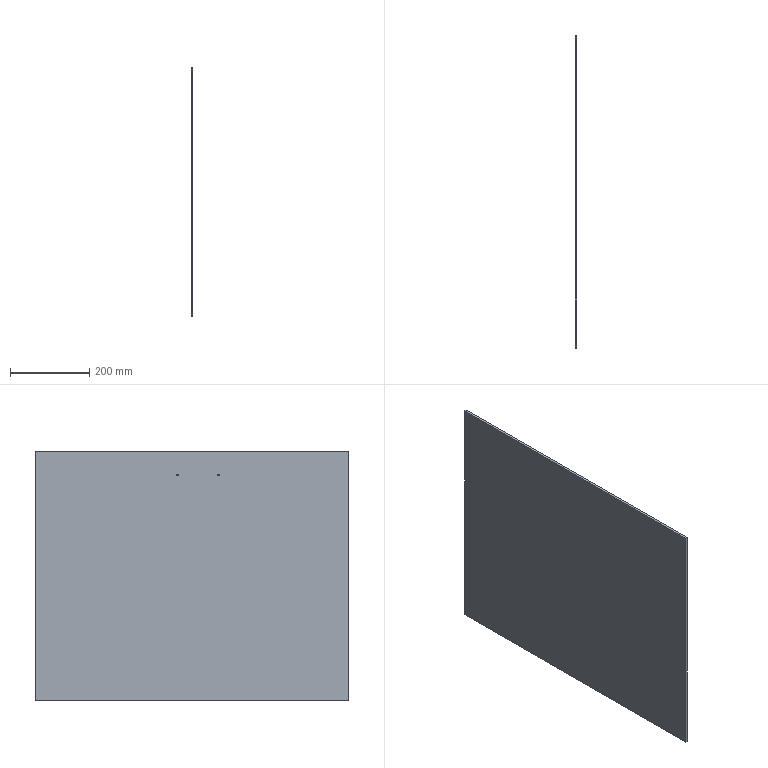Part | STEP file | 08-07 Guard maintenance door | 1 solid | 10 faces | box 5 x 790 x 630 mm | volume 2488341 mm3 | plane 6 | cylinder 4 | commonest cylinder face diameters 4.5 x4
STEP:
#1=CARTESIAN_POINT('',(0.,0.,0.));
#2=DIRECTION('',(0.,0.,1.));
#3=DIRECTION('',(1.,0.,0.));
#4=AXIS2_PLACEMENT_3D('',#1,#2,#3);
#5=CARTESIAN_POINT('',(0.,328.,-62.25));
#6=VERTEX_POINT('',#5);
#7=CARTESIAN_POINT('',(5.,328.,-62.25));
#8=VERTEX_POINT('',#7);
#9=CARTESIAN_POINT('',(0.,328.,-62.25));
#10=DIRECTION('',(1.,0.,0.));
#11=VECTOR('',#10,1.);
#12=LINE('',#9,#11);
#13=CARTESIAN_POINT('',(0.,328.,-60.));
#14=DIRECTION('',(1.,0.,0.));
#15=DIRECTION('',(0.,0.,-1.));
#16=AXIS2_PLACEMENT_3D('',#13,#14,#15);
#17=CYLINDRICAL_SURFACE('',#16,2.25);
#18=CARTESIAN_POINT('',(6.283,0.));
#19=DIRECTION('',(0.,1.));
#20=VECTOR('',#19,1.);
#21=LINE('',#18,#20);
#22=(GEOMETRIC_REPRESENTATION_CONTEXT(2)PARAMETRIC_REPRESENTATION_CONTEXT()REPRESENTATION_CONTEXT('',''));
#23=DEFINITIONAL_REPRESENTATION('',(#21),#22);
#24=PCURVE('',#17,#23);
#25=CARTESIAN_POINT('',(0.,328.,-60.));
#26=DIRECTION('',(1.,0.,0.));
#27=DIRECTION('',(0.,0.,-1.));
#28=AXIS2_PLACEMENT_3D('',#25,#26,#27);
#29=CYLINDRICAL_SURFACE('',#28,2.25);
#30=CARTESIAN_POINT('',(0.,0.));
#31=DIRECTION('',(0.,1.));
#32=VECTOR('',#31,1.);
#33=LINE('',#30,#32);
#34=(GEOMETRIC_REPRESENTATION_CONTEXT(2)PARAMETRIC_REPRESENTATION_CONTEXT()REPRESENTATION_CONTEXT('',''));
#35=DEFINITIONAL_REPRESENTATION('',(#33),#34);
#36=PCURVE('',#29,#35);
#37=SURFACE_CURVE('',#12,(#24,#36),.PCURVE_S1.);
#38=EDGE_CURVE('',#6,#8,#37,.T.);
#39=ORIENTED_EDGE('',*,*,#38,.T.);
#40=CARTESIAN_POINT('',(5.,328.,-57.75));
#41=VERTEX_POINT('',#40);
#42=CARTESIAN_POINT('',(5.,328.,-60.));
#43=DIRECTION('',(1.,0.,0.));
#44=DIRECTION('',(0.,0.,-1.));
#45=AXIS2_PLACEMENT_3D('',#42,#43,#44);
#46=CIRCLE('',#45,2.25);
#47=CARTESIAN_POINT('',(0.,5.));
#48=DIRECTION('',(1.,0.));
#49=VECTOR('',#48,1.);
#50=LINE('',#47,#49);
#51=(GEOMETRIC_REPRESENTATION_CONTEXT(2)PARAMETRIC_REPRESENTATION_CONTEXT()REPRESENTATION_CONTEXT('',''));
#52=DEFINITIONAL_REPRESENTATION('',(#50),#51);
#53=PCURVE('',#17,#52);
#54=CARTESIAN_POINT('',(5.,0.,-630.));
#55=DIRECTION('',(-1.,0.,0.));
#56=DIRECTION('',(0.,0.,1.));
#57=AXIS2_PLACEMENT_3D('',#54,#55,#56);
#58=PLANE('',#57);
#59=CARTESIAN_POINT('',(567.75,328.));
#60=CARTESIAN_POINT('',(567.75,331.897));
#61=CARTESIAN_POINT('',(571.125,329.949));
#62=CARTESIAN_POINT('',(574.5,328.));
#63=CARTESIAN_POINT('',(571.125,326.051));
#64=CARTESIAN_POINT('',(567.75,324.103));
#65=CARTESIAN_POINT('',(567.75,328.));
#66=(BOUNDED_CURVE()B_SPLINE_CURVE(2,(#59,#60,#61,#62,#63,#64,#65),.UNSPECIFIED.,.T.,.F.)B_SPLINE_CURVE_WITH_KNOTS((1,2,2,2,2,1),(-2.094,0.,2.094,4.189,6.283,8.378),.UNSPECIFIED.)CURVE()GEOMETRIC_REPRESENTATION_ITEM()RATIONAL_B_SPLINE_CURVE((1.,0.5,1.,0.5,1.,0.5,1.))REPRESENTATION_ITEM(''));
#67=(GEOMETRIC_REPRESENTATION_CONTEXT(2)PARAMETRIC_REPRESENTATION_CONTEXT()REPRESENTATION_CONTEXT('',''));
#68=DEFINITIONAL_REPRESENTATION('',(#66),#67);
#69=PCURVE('',#58,#68);
#70=SURFACE_CURVE('',#46,(#53,#69),.PCURVE_S1.);
#71=EDGE_CURVE('',#41,#8,#70,.T.);
#72=ORIENTED_EDGE('',*,*,#71,.F.);
#73=CARTESIAN_POINT('',(0.,328.,-57.75));
#74=VERTEX_POINT('',#73);
#75=CARTESIAN_POINT('',(0.,328.,-57.75));
#76=DIRECTION('',(1.,0.,0.));
#77=VECTOR('',#76,1.);
#78=LINE('',#75,#77);
#79=CARTESIAN_POINT('',(3.142,0.));
#80=DIRECTION('',(0.,1.));
#81=VECTOR('',#80,1.);
#82=LINE('',#79,#81);
#83=(GEOMETRIC_REPRESENTATION_CONTEXT(2)PARAMETRIC_REPRESENTATION_CONTEXT()REPRESENTATION_CONTEXT('',''));
#84=DEFINITIONAL_REPRESENTATION('',(#82),#83);
#85=PCURVE('',#17,#84);
#86=CARTESIAN_POINT('',(3.142,0.));
#87=DIRECTION('',(0.,1.));
#88=VECTOR('',#87,1.);
#89=LINE('',#86,#88);
#90=(GEOMETRIC_REPRESENTATION_CONTEXT(2)PARAMETRIC_REPRESENTATION_CONTEXT()REPRESENTATION_CONTEXT('',''));
#91=DEFINITIONAL_REPRESENTATION('',(#89),#90);
#92=PCURVE('',#29,#91);
#93=SURFACE_CURVE('',#78,(#85,#92),.PCURVE_S1.);
#94=EDGE_CURVE('',#74,#41,#93,.T.);
#95=ORIENTED_EDGE('',*,*,#94,.F.);
#96=CARTESIAN_POINT('',(0.,328.,-60.));
#97=DIRECTION('',(-1.,0.,0.));
#98=DIRECTION('',(0.,0.,-1.));
#99=AXIS2_PLACEMENT_3D('',#96,#97,#98);
#100=CIRCLE('',#99,2.25);
#101=CARTESIAN_POINT('',(6.283,0.));
#102=DIRECTION('',(-1.,0.));
#103=VECTOR('',#102,1.);
#104=LINE('',#101,#103);
#105=(GEOMETRIC_REPRESENTATION_CONTEXT(2)PARAMETRIC_REPRESENTATION_CONTEXT()REPRESENTATION_CONTEXT('',''));
#106=DEFINITIONAL_REPRESENTATION('',(#104),#105);
#107=PCURVE('',#17,#106);
#108=CARTESIAN_POINT('',(0.,0.,-630.));
#109=DIRECTION('',(-1.,0.,0.));
#110=DIRECTION('',(0.,0.,1.));
#111=AXIS2_PLACEMENT_3D('',#108,#109,#110);
#112=PLANE('',#111);
#113=CARTESIAN_POINT('',(570.,328.));
#114=DIRECTION('',(-1.,0.));
#115=AXIS2_PLACEMENT_2D('',#113,#114);
#116=CIRCLE('',#115,2.25);
#117=(GEOMETRIC_REPRESENTATION_CONTEXT(2)PARAMETRIC_REPRESENTATION_CONTEXT()REPRESENTATION_CONTEXT('',''));
#118=DEFINITIONAL_REPRESENTATION('',(#116),#117);
#119=PCURVE('',#112,#118);
#120=SURFACE_CURVE('',#100,(#107,#119),.PCURVE_S1.);
#121=EDGE_CURVE('',#6,#74,#120,.T.);
#122=ORIENTED_EDGE('',*,*,#121,.F.);
#123=EDGE_LOOP('',(#39,#72,#95,#122));
#124=FACE_BOUND('',#123,.F.);
#125=ADVANCED_FACE('',(#124),#17,.F.);
#126=CARTESIAN_POINT('',(0.,432.,-62.25));
#127=VERTEX_POINT('',#126);
#128=CARTESIAN_POINT('',(5.,432.,-62.25));
#129=VERTEX_POINT('',#128);
#130=CARTESIAN_POINT('',(0.,432.,-62.25));
#131=DIRECTION('',(1.,0.,0.));
#132=VECTOR('',#131,1.);
#133=LINE('',#130,#132);
#134=CARTESIAN_POINT('',(0.,432.,-60.));
#135=DIRECTION('',(1.,0.,0.));
#136=DIRECTION('',(0.,0.,-1.));
#137=AXIS2_PLACEMENT_3D('',#134,#135,#136);
#138=CYLINDRICAL_SURFACE('',#137,2.25);
#139=CARTESIAN_POINT('',(6.283,0.));
#140=DIRECTION('',(0.,1.));
#141=VECTOR('',#140,1.);
#142=LINE('',#139,#141);
#143=(GEOMETRIC_REPRESENTATION_CONTEXT(2)PARAMETRIC_REPRESENTATION_CONTEXT()REPRESENTATION_CONTEXT('',''));
#144=DEFINITIONAL_REPRESENTATION('',(#142),#143);
#145=PCURVE('',#138,#144);
#146=CARTESIAN_POINT('',(0.,432.,-60.));
#147=DIRECTION('',(1.,0.,0.));
#148=DIRECTION('',(0.,0.,-1.));
#149=AXIS2_PLACEMENT_3D('',#146,#147,#148);
#150=CYLINDRICAL_SURFACE('',#149,2.25);
#151=CARTESIAN_POINT('',(0.,0.));
#152=DIRECTION('',(0.,1.));
#153=VECTOR('',#152,1.);
#154=LINE('',#151,#153);
#155=(GEOMETRIC_REPRESENTATION_CONTEXT(2)PARAMETRIC_REPRESENTATION_CONTEXT()REPRESENTATION_CONTEXT('',''));
#156=DEFINITIONAL_REPRESENTATION('',(#154),#155);
#157=PCURVE('',#150,#156);
#158=SURFACE_CURVE('',#133,(#145,#157),.PCURVE_S1.);
#159=EDGE_CURVE('',#127,#129,#158,.T.);
#160=ORIENTED_EDGE('',*,*,#159,.T.);
#161=CARTESIAN_POINT('',(5.,432.,-57.75));
#162=VERTEX_POINT('',#161);
#163=CARTESIAN_POINT('',(5.,432.,-60.));
#164=DIRECTION('',(1.,0.,0.));
#165=DIRECTION('',(0.,0.,-1.));
#166=AXIS2_PLACEMENT_3D('',#163,#164,#165);
#167=CIRCLE('',#166,2.25);
#168=CARTESIAN_POINT('',(0.,5.));
#169=DIRECTION('',(1.,0.));
#170=VECTOR('',#169,1.);
#171=LINE('',#168,#170);
#172=(GEOMETRIC_REPRESENTATION_CONTEXT(2)PARAMETRIC_REPRESENTATION_CONTEXT()REPRESENTATION_CONTEXT('',''));
#173=DEFINITIONAL_REPRESENTATION('',(#171),#172);
#174=PCURVE('',#138,#173);
#175=CARTESIAN_POINT('',(567.75,432.));
#176=CARTESIAN_POINT('',(567.75,435.897));
#177=CARTESIAN_POINT('',(571.125,433.949));
#178=CARTESIAN_POINT('',(574.5,432.));
#179=CARTESIAN_POINT('',(571.125,430.051));
#180=CARTESIAN_POINT('',(567.75,428.103));
#181=CARTESIAN_POINT('',(567.75,432.));
#182=(BOUNDED_CURVE()B_SPLINE_CURVE(2,(#175,#176,#177,#178,#179,#180,#181),.UNSPECIFIED.,.T.,.F.)B_SPLINE_CURVE_WITH_KNOTS((1,2,2,2,2,1),(-2.094,0.,2.094,4.189,6.283,8.378),.UNSPECIFIED.)CURVE()GEOMETRIC_REPRESENTATION_ITEM()RATIONAL_B_SPLINE_CURVE((1.,0.5,1.,0.5,1.,0.5,1.))REPRESENTATION_ITEM(''));
#183=(GEOMETRIC_REPRESENTATION_CONTEXT(2)PARAMETRIC_REPRESENTATION_CONTEXT()REPRESENTATION_CONTEXT('',''));
#184=DEFINITIONAL_REPRESENTATION('',(#182),#183);
#185=PCURVE('',#58,#184);
#186=SURFACE_CURVE('',#167,(#174,#185),.PCURVE_S1.);
#187=EDGE_CURVE('',#162,#129,#186,.T.);
#188=ORIENTED_EDGE('',*,*,#187,.F.);
#189=CARTESIAN_POINT('',(0.,432.,-57.75));
#190=VERTEX_POINT('',#189);
#191=CARTESIAN_POINT('',(0.,432.,-57.75));
#192=DIRECTION('',(1.,0.,0.));
#193=VECTOR('',#192,1.);
#194=LINE('',#191,#193);
#195=CARTESIAN_POINT('',(3.142,0.));
#196=DIRECTION('',(0.,1.));
#197=VECTOR('',#196,1.);
#198=LINE('',#195,#197);
#199=(GEOMETRIC_REPRESENTATION_CONTEXT(2)PARAMETRIC_REPRESENTATION_CONTEXT()REPRESENTATION_CONTEXT('',''));
#200=DEFINITIONAL_REPRESENTATION('',(#198),#199);
#201=PCURVE('',#138,#200);
#202=CARTESIAN_POINT('',(3.142,0.));
#203=DIRECTION('',(0.,1.));
#204=VECTOR('',#203,1.);
#205=LINE('',#202,#204);
#206=(GEOMETRIC_REPRESENTATION_CONTEXT(2)PARAMETRIC_REPRESENTATION_CONTEXT()REPRESENTATION_CONTEXT('',''));
#207=DEFINITIONAL_REPRESENTATION('',(#205),#206);
#208=PCURVE('',#150,#207);
#209=SURFACE_CURVE('',#194,(#201,#208),.PCURVE_S1.);
#210=EDGE_CURVE('',#190,#162,#209,.T.);
#211=ORIENTED_EDGE('',*,*,#210,.F.);
#212=CARTESIAN_POINT('',(0.,432.,-60.));
#213=DIRECTION('',(1.,0.,0.));
#214=DIRECTION('',(0.,0.,-1.));
#215=AXIS2_PLACEMENT_3D('',#212,#213,#214);
#216=CIRCLE('',#215,2.25);
#217=CARTESIAN_POINT('',(0.,0.));
#218=DIRECTION('',(1.,0.));
#219=VECTOR('',#218,1.);
#220=LINE('',#217,#219);
#221=(GEOMETRIC_REPRESENTATION_CONTEXT(2)PARAMETRIC_REPRESENTATION_CONTEXT()REPRESENTATION_CONTEXT('',''));
#222=DEFINITIONAL_REPRESENTATION('',(#220),#221);
#223=PCURVE('',#138,#222);
#224=CARTESIAN_POINT('',(567.75,432.));
#225=CARTESIAN_POINT('',(567.75,435.897));
#226=CARTESIAN_POINT('',(571.125,433.949));
#227=CARTESIAN_POINT('',(574.5,432.));
#228=CARTESIAN_POINT('',(571.125,430.051));
#229=CARTESIAN_POINT('',(567.75,428.103));
#230=CARTESIAN_POINT('',(567.75,432.));
#231=(BOUNDED_CURVE()B_SPLINE_CURVE(2,(#224,#225,#226,#227,#228,#229,#230),.UNSPECIFIED.,.T.,.F.)B_SPLINE_CURVE_WITH_KNOTS((1,2,2,2,2,1),(-2.094,0.,2.094,4.189,6.283,8.378),.UNSPECIFIED.)CURVE()GEOMETRIC_REPRESENTATION_ITEM()RATIONAL_B_SPLINE_CURVE((1.,0.5,1.,0.5,1.,0.5,1.))REPRESENTATION_ITEM(''));
#232=(GEOMETRIC_REPRESENTATION_CONTEXT(2)PARAMETRIC_REPRESENTATION_CONTEXT()REPRESENTATION_CONTEXT('',''));
#233=DEFINITIONAL_REPRESENTATION('',(#231),#232);
#234=PCURVE('',#112,#233);
#235=SURFACE_CURVE('',#216,(#223,#234),.PCURVE_S1.);
#236=EDGE_CURVE('',#190,#127,#235,.T.);
#237=ORIENTED_EDGE('',*,*,#236,.T.);
#238=EDGE_LOOP('',(#160,#188,#211,#237));
#239=FACE_BOUND('',#238,.F.);
#240=ADVANCED_FACE('',(#239),#138,.F.);
#241=CARTESIAN_POINT('',(5.,328.,-60.));
#242=DIRECTION('',(1.,0.,0.));
#243=DIRECTION('',(0.,0.,-1.));
#244=AXIS2_PLACEMENT_3D('',#241,#242,#243);
#245=CIRCLE('',#244,2.25);
#246=CARTESIAN_POINT('',(0.,5.));
#247=DIRECTION('',(1.,0.));
#248=VECTOR('',#247,1.);
#249=LINE('',#246,#248);
#250=(GEOMETRIC_REPRESENTATION_CONTEXT(2)PARAMETRIC_REPRESENTATION_CONTEXT()REPRESENTATION_CONTEXT('',''));
#251=DEFINITIONAL_REPRESENTATION('',(#249),#250);
#252=PCURVE('',#29,#251);
#253=CARTESIAN_POINT('',(567.75,328.));
#254=CARTESIAN_POINT('',(567.75,331.897));
#255=CARTESIAN_POINT('',(571.125,329.949));
#256=CARTESIAN_POINT('',(574.5,328.));
#257=CARTESIAN_POINT('',(571.125,326.051));
#258=CARTESIAN_POINT('',(567.75,324.103));
#259=CARTESIAN_POINT('',(567.75,328.));
#260=(BOUNDED_CURVE()B_SPLINE_CURVE(2,(#253,#254,#255,#256,#257,#258,#259),.UNSPECIFIED.,.T.,.F.)B_SPLINE_CURVE_WITH_KNOTS((1,2,2,2,2,1),(-2.094,0.,2.094,4.189,6.283,8.378),.UNSPECIFIED.)CURVE()GEOMETRIC_REPRESENTATION_ITEM()RATIONAL_B_SPLINE_CURVE((1.,0.5,1.,0.5,1.,0.5,1.))REPRESENTATION_ITEM(''));
#261=(GEOMETRIC_REPRESENTATION_CONTEXT(2)PARAMETRIC_REPRESENTATION_CONTEXT()REPRESENTATION_CONTEXT('',''));
#262=DEFINITIONAL_REPRESENTATION('',(#260),#261);
#263=PCURVE('',#58,#262);
#264=SURFACE_CURVE('',#245,(#252,#263),.PCURVE_S1.);
#265=EDGE_CURVE('',#8,#41,#264,.T.);
#266=ORIENTED_EDGE('',*,*,#265,.F.);
#267=ORIENTED_EDGE('',*,*,#38,.F.);
#268=CARTESIAN_POINT('',(0.,328.,-60.));
#269=DIRECTION('',(-1.,0.,0.));
#270=DIRECTION('',(0.,0.,-1.));
#271=AXIS2_PLACEMENT_3D('',#268,#269,#270);
#272=CIRCLE('',#271,2.25);
#273=CARTESIAN_POINT('',(6.283,0.));
#274=DIRECTION('',(-1.,0.));
#275=VECTOR('',#274,1.);
#276=LINE('',#273,#275);
#277=(GEOMETRIC_REPRESENTATION_CONTEXT(2)PARAMETRIC_REPRESENTATION_CONTEXT()REPRESENTATION_CONTEXT('',''));
#278=DEFINITIONAL_REPRESENTATION('',(#276),#277);
#279=PCURVE('',#29,#278);
#280=CARTESIAN_POINT('',(570.,328.));
#281=DIRECTION('',(-1.,0.));
#282=AXIS2_PLACEMENT_2D('',#280,#281);
#283=CIRCLE('',#282,2.25);
#284=(GEOMETRIC_REPRESENTATION_CONTEXT(2)PARAMETRIC_REPRESENTATION_CONTEXT()REPRESENTATION_CONTEXT('',''));
#285=DEFINITIONAL_REPRESENTATION('',(#283),#284);
#286=PCURVE('',#112,#285);
#287=SURFACE_CURVE('',#272,(#279,#286),.PCURVE_S1.);
#288=EDGE_CURVE('',#74,#6,#287,.T.);
#289=ORIENTED_EDGE('',*,*,#288,.F.);
#290=ORIENTED_EDGE('',*,*,#94,.T.);
#291=EDGE_LOOP('',(#266,#267,#289,#290));
#292=FACE_BOUND('',#291,.F.);
#293=ADVANCED_FACE('',(#292),#29,.F.);
#294=CARTESIAN_POINT('',(5.,432.,-60.));
#295=DIRECTION('',(1.,0.,0.));
#296=DIRECTION('',(0.,0.,-1.));
#297=AXIS2_PLACEMENT_3D('',#294,#295,#296);
#298=CIRCLE('',#297,2.25);
#299=CARTESIAN_POINT('',(567.75,432.));
#300=CARTESIAN_POINT('',(567.75,435.897));
#301=CARTESIAN_POINT('',(571.125,433.949));
#302=CARTESIAN_POINT('',(574.5,432.));
#303=CARTESIAN_POINT('',(571.125,430.051));
#304=CARTESIAN_POINT('',(567.75,428.103));
#305=CARTESIAN_POINT('',(567.75,432.));
#306=(BOUNDED_CURVE()B_SPLINE_CURVE(2,(#299,#300,#301,#302,#303,#304,#305),.UNSPECIFIED.,.T.,.F.)B_SPLINE_CURVE_WITH_KNOTS((1,2,2,2,2,1),(-2.094,0.,2.094,4.189,6.283,8.378),.UNSPECIFIED.)CURVE()GEOMETRIC_REPRESENTATION_ITEM()RATIONAL_B_SPLINE_CURVE((1.,0.5,1.,0.5,1.,0.5,1.))REPRESENTATION_ITEM(''));
#307=(GEOMETRIC_REPRESENTATION_CONTEXT(2)PARAMETRIC_REPRESENTATION_CONTEXT()REPRESENTATION_CONTEXT('',''));
#308=DEFINITIONAL_REPRESENTATION('',(#306),#307);
#309=PCURVE('',#58,#308);
#310=CARTESIAN_POINT('',(0.,5.));
#311=DIRECTION('',(1.,0.));
#312=VECTOR('',#311,1.);
#313=LINE('',#310,#312);
#314=(GEOMETRIC_REPRESENTATION_CONTEXT(2)PARAMETRIC_REPRESENTATION_CONTEXT()REPRESENTATION_CONTEXT('',''));
#315=DEFINITIONAL_REPRESENTATION('',(#313),#314);
#316=PCURVE('',#150,#315);
#317=SURFACE_CURVE('',#298,(#309,#316),.PCURVE_S1.);
#318=EDGE_CURVE('',#129,#162,#317,.T.);
#319=ORIENTED_EDGE('',*,*,#318,.F.);
#320=ORIENTED_EDGE('',*,*,#187,.F.);
#321=EDGE_LOOP('',(#319,#320));
#322=FACE_BOUND('',#321,.T.);
#323=ORIENTED_EDGE('',*,*,#265,.F.);
#324=ORIENTED_EDGE('',*,*,#71,.F.);
#325=EDGE_LOOP('',(#323,#324));
#326=FACE_BOUND('',#325,.T.);
#327=CARTESIAN_POINT('',(5.,0.,-630.));
#328=VERTEX_POINT('',#327);
#329=CARTESIAN_POINT('',(5.,0.,0.));
#330=VERTEX_POINT('',#329);
#331=CARTESIAN_POINT('',(5.,0.,-315.));
#332=DIRECTION('',(0.,0.,1.));
#333=VECTOR('',#332,1.);
#334=LINE('',#331,#333);
#335=CARTESIAN_POINT('',(315.,0.));
#336=DIRECTION('',(1.,0.));
#337=VECTOR('',#336,1.);
#338=LINE('',#335,#337);
#339=(GEOMETRIC_REPRESENTATION_CONTEXT(2)PARAMETRIC_REPRESENTATION_CONTEXT()REPRESENTATION_CONTEXT('',''));
#340=DEFINITIONAL_REPRESENTATION('',(#338),#339);
#341=PCURVE('',#58,#340);
#342=CARTESIAN_POINT('',(0.,0.,-630.));
#343=DIRECTION('',(0.,1.,0.));
#344=DIRECTION('',(0.,0.,1.));
#345=AXIS2_PLACEMENT_3D('',#342,#343,#344);
#346=PLANE('',#345);
#347=CARTESIAN_POINT('',(315.,5.));
#348=DIRECTION('',(1.,0.));
#349=VECTOR('',#348,1.);
#350=LINE('',#347,#349);
#351=(GEOMETRIC_REPRESENTATION_CONTEXT(2)PARAMETRIC_REPRESENTATION_CONTEXT()REPRESENTATION_CONTEXT('',''));
#352=DEFINITIONAL_REPRESENTATION('',(#350),#351);
#353=PCURVE('',#346,#352);
#354=SURFACE_CURVE('',#334,(#341,#353),.PCURVE_S1.);
#355=EDGE_CURVE('',#328,#330,#354,.T.);
#356=ORIENTED_EDGE('',*,*,#355,.F.);
#357=CARTESIAN_POINT('',(5.,790.,-630.));
#358=VERTEX_POINT('',#357);
#359=CARTESIAN_POINT('',(5.,395.,-630.));
#360=DIRECTION('',(0.,-1.,0.));
#361=VECTOR('',#360,1.);
#362=LINE('',#359,#361);
#363=CARTESIAN_POINT('',(0.,395.));
#364=DIRECTION('',(0.,-1.));
#365=VECTOR('',#364,1.);
#366=LINE('',#363,#365);
#367=(GEOMETRIC_REPRESENTATION_CONTEXT(2)PARAMETRIC_REPRESENTATION_CONTEXT()REPRESENTATION_CONTEXT('',''));
#368=DEFINITIONAL_REPRESENTATION('',(#366),#367);
#369=PCURVE('',#58,#368);
#370=CARTESIAN_POINT('',(0.,0.,-630.));
#371=DIRECTION('',(0.,0.,1.));
#372=DIRECTION('',(1.,0.,0.));
#373=AXIS2_PLACEMENT_3D('',#370,#371,#372);
#374=PLANE('',#373);
#375=CARTESIAN_POINT('',(5.,395.));
#376=DIRECTION('',(0.,-1.));
#377=VECTOR('',#376,1.);
#378=LINE('',#375,#377);
#379=(GEOMETRIC_REPRESENTATION_CONTEXT(2)PARAMETRIC_REPRESENTATION_CONTEXT()REPRESENTATION_CONTEXT('',''));
#380=DEFINITIONAL_REPRESENTATION('',(#378),#379);
#381=PCURVE('',#374,#380);
#382=SURFACE_CURVE('',#362,(#369,#381),.PCURVE_S1.);
#383=EDGE_CURVE('',#358,#328,#382,.T.);
#384=ORIENTED_EDGE('',*,*,#383,.F.);
#385=CARTESIAN_POINT('',(5.,790.,0.));
#386=VERTEX_POINT('',#385);
#387=CARTESIAN_POINT('',(5.,790.,-315.));
#388=DIRECTION('',(0.,0.,-1.));
#389=VECTOR('',#388,1.);
#390=LINE('',#387,#389);
#391=CARTESIAN_POINT('',(315.,790.));
#392=DIRECTION('',(-1.,0.));
#393=VECTOR('',#392,1.);
#394=LINE('',#391,#393);
#395=(GEOMETRIC_REPRESENTATION_CONTEXT(2)PARAMETRIC_REPRESENTATION_CONTEXT()REPRESENTATION_CONTEXT('',''));
#396=DEFINITIONAL_REPRESENTATION('',(#394),#395);
#397=PCURVE('',#58,#396);
#398=CARTESIAN_POINT('',(0.,790.,0.));
#399=DIRECTION('',(0.,-1.,0.));
#400=DIRECTION('',(0.,0.,-1.));
#401=AXIS2_PLACEMENT_3D('',#398,#399,#400);
#402=PLANE('',#401);
#403=CARTESIAN_POINT('',(315.,5.));
#404=DIRECTION('',(1.,0.));
#405=VECTOR('',#404,1.);
#406=LINE('',#403,#405);
#407=(GEOMETRIC_REPRESENTATION_CONTEXT(2)PARAMETRIC_REPRESENTATION_CONTEXT()REPRESENTATION_CONTEXT('',''));
#408=DEFINITIONAL_REPRESENTATION('',(#406),#407);
#409=PCURVE('',#402,#408);
#410=SURFACE_CURVE('',#390,(#397,#409),.PCURVE_S1.);
#411=EDGE_CURVE('',#386,#358,#410,.T.);
#412=ORIENTED_EDGE('',*,*,#411,.F.);
#413=CARTESIAN_POINT('',(5.,395.,0.));
#414=DIRECTION('',(0.,1.,0.));
#415=VECTOR('',#414,1.);
#416=LINE('',#413,#415);
#417=CARTESIAN_POINT('',(630.,395.));
#418=DIRECTION('',(0.,1.));
#419=VECTOR('',#418,1.);
#420=LINE('',#417,#419);
#421=(GEOMETRIC_REPRESENTATION_CONTEXT(2)PARAMETRIC_REPRESENTATION_CONTEXT()REPRESENTATION_CONTEXT('',''));
#422=DEFINITIONAL_REPRESENTATION('',(#420),#421);
#423=PCURVE('',#58,#422);
#424=CARTESIAN_POINT('',(5.,0.,0.));
#425=DIRECTION('',(0.,0.,-1.));
#426=DIRECTION('',(-1.,0.,0.));
#427=AXIS2_PLACEMENT_3D('',#424,#425,#426);
#428=PLANE('',#427);
#429=CARTESIAN_POINT('',(0.,395.));
#430=DIRECTION('',(0.,1.));
#431=VECTOR('',#430,1.);
#432=LINE('',#429,#431);
#433=(GEOMETRIC_REPRESENTATION_CONTEXT(2)PARAMETRIC_REPRESENTATION_CONTEXT()REPRESENTATION_CONTEXT('',''));
#434=DEFINITIONAL_REPRESENTATION('',(#432),#433);
#435=PCURVE('',#428,#434);
#436=SURFACE_CURVE('',#416,(#423,#435),.PCURVE_S1.);
#437=EDGE_CURVE('',#330,#386,#436,.T.);
#438=ORIENTED_EDGE('',*,*,#437,.F.);
#439=EDGE_LOOP('',(#356,#384,#412,#438));
#440=FACE_BOUND('',#439,.T.);
#441=ADVANCED_FACE('',(#322,#326,#440),#58,.F.);
#442=CARTESIAN_POINT('',(0.,432.,-60.));
#443=DIRECTION('',(1.,0.,0.));
#444=DIRECTION('',(0.,0.,-1.));
#445=AXIS2_PLACEMENT_3D('',#442,#443,#444);
#446=CIRCLE('',#445,2.25);
#447=CARTESIAN_POINT('',(567.75,432.));
#448=CARTESIAN_POINT('',(567.75,435.897));
#449=CARTESIAN_POINT('',(571.125,433.949));
#450=CARTESIAN_POINT('',(574.5,432.));
#451=CARTESIAN_POINT('',(571.125,430.051));
#452=CARTESIAN_POINT('',(567.75,428.103));
#453=CARTESIAN_POINT('',(567.75,432.));
#454=(BOUNDED_CURVE()B_SPLINE_CURVE(2,(#447,#448,#449,#450,#451,#452,#453),.UNSPECIFIED.,.T.,.F.)B_SPLINE_CURVE_WITH_KNOTS((1,2,2,2,2,1),(-2.094,0.,2.094,4.189,6.283,8.378),.UNSPECIFIED.)CURVE()GEOMETRIC_REPRESENTATION_ITEM()RATIONAL_B_SPLINE_CURVE((1.,0.5,1.,0.5,1.,0.5,1.))REPRESENTATION_ITEM(''));
#455=(GEOMETRIC_REPRESENTATION_CONTEXT(2)PARAMETRIC_REPRESENTATION_CONTEXT()REPRESENTATION_CONTEXT('',''));
#456=DEFINITIONAL_REPRESENTATION('',(#454),#455);
#457=PCURVE('',#112,#456);
#458=CARTESIAN_POINT('',(0.,0.));
#459=DIRECTION('',(1.,0.));
#460=VECTOR('',#459,1.);
#461=LINE('',#458,#460);
#462=(GEOMETRIC_REPRESENTATION_CONTEXT(2)PARAMETRIC_REPRESENTATION_CONTEXT()REPRESENTATION_CONTEXT('',''));
#463=DEFINITIONAL_REPRESENTATION('',(#461),#462);
#464=PCURVE('',#150,#463);
#465=SURFACE_CURVE('',#446,(#457,#464),.PCURVE_S1.);
#466=EDGE_CURVE('',#127,#190,#465,.T.);
#467=ORIENTED_EDGE('',*,*,#466,.T.);
#468=ORIENTED_EDGE('',*,*,#236,.T.);
#469=EDGE_LOOP('',(#467,#468));
#470=FACE_BOUND('',#469,.T.);
#471=ORIENTED_EDGE('',*,*,#121,.F.);
#472=ORIENTED_EDGE('',*,*,#288,.F.);
#473=EDGE_LOOP('',(#471,#472));
#474=FACE_BOUND('',#473,.T.);
#475=CARTESIAN_POINT('',(0.,790.,-630.));
#476=VERTEX_POINT('',#475);
#477=CARTESIAN_POINT('',(0.,0.,-630.));
#478=VERTEX_POINT('',#477);
#479=CARTESIAN_POINT('',(0.,395.,-630.));
#480=DIRECTION('',(0.,-1.,0.));
#481=VECTOR('',#480,1.);
#482=LINE('',#479,#481);
#483=CARTESIAN_POINT('',(0.,395.));
#484=DIRECTION('',(0.,-1.));
#485=VECTOR('',#484,1.);
#486=LINE('',#483,#485);
#487=(GEOMETRIC_REPRESENTATION_CONTEXT(2)PARAMETRIC_REPRESENTATION_CONTEXT()REPRESENTATION_CONTEXT('',''));
#488=DEFINITIONAL_REPRESENTATION('',(#486),#487);
#489=PCURVE('',#112,#488);
#490=CARTESIAN_POINT('',(0.,395.));
#491=DIRECTION('',(0.,-1.));
#492=VECTOR('',#491,1.);
#493=LINE('',#490,#492);
#494=(GEOMETRIC_REPRESENTATION_CONTEXT(2)PARAMETRIC_REPRESENTATION_CONTEXT()REPRESENTATION_CONTEXT('',''));
#495=DEFINITIONAL_REPRESENTATION('',(#493),#494);
#496=PCURVE('',#374,#495);
#497=SURFACE_CURVE('',#482,(#489,#496),.PCURVE_S1.);
#498=EDGE_CURVE('',#476,#478,#497,.T.);
#499=ORIENTED_EDGE('',*,*,#498,.T.);
#500=CARTESIAN_POINT('',(0.,0.,0.));
#501=VERTEX_POINT('',#500);
#502=CARTESIAN_POINT('',(0.,0.,-315.));
#503=DIRECTION('',(0.,0.,1.));
#504=VECTOR('',#503,1.);
#505=LINE('',#502,#504);
#506=CARTESIAN_POINT('',(315.,0.));
#507=DIRECTION('',(1.,0.));
#508=VECTOR('',#507,1.);
#509=LINE('',#506,#508);
#510=(GEOMETRIC_REPRESENTATION_CONTEXT(2)PARAMETRIC_REPRESENTATION_CONTEXT()REPRESENTATION_CONTEXT('',''));
#511=DEFINITIONAL_REPRESENTATION('',(#509),#510);
#512=PCURVE('',#112,#511);
#513=CARTESIAN_POINT('',(315.,0.));
#514=DIRECTION('',(1.,0.));
#515=VECTOR('',#514,1.);
#516=LINE('',#513,#515);
#517=(GEOMETRIC_REPRESENTATION_CONTEXT(2)PARAMETRIC_REPRESENTATION_CONTEXT()REPRESENTATION_CONTEXT('',''));
#518=DEFINITIONAL_REPRESENTATION('',(#516),#517);
#519=PCURVE('',#346,#518);
#520=SURFACE_CURVE('',#505,(#512,#519),.PCURVE_S1.);
#521=EDGE_CURVE('',#478,#501,#520,.T.);
#522=ORIENTED_EDGE('',*,*,#521,.T.);
#523=CARTESIAN_POINT('',(0.,790.,0.));
#524=VERTEX_POINT('',#523);
#525=CARTESIAN_POINT('',(0.,395.,0.));
#526=DIRECTION('',(0.,1.,0.));
#527=VECTOR('',#526,1.);
#528=LINE('',#525,#527);
#529=CARTESIAN_POINT('',(630.,395.));
#530=DIRECTION('',(0.,1.));
#531=VECTOR('',#530,1.);
#532=LINE('',#529,#531);
#533=(GEOMETRIC_REPRESENTATION_CONTEXT(2)PARAMETRIC_REPRESENTATION_CONTEXT()REPRESENTATION_CONTEXT('',''));
#534=DEFINITIONAL_REPRESENTATION('',(#532),#533);
#535=PCURVE('',#112,#534);
#536=CARTESIAN_POINT('',(5.,395.));
#537=DIRECTION('',(0.,1.));
#538=VECTOR('',#537,1.);
#539=LINE('',#536,#538);
#540=(GEOMETRIC_REPRESENTATION_CONTEXT(2)PARAMETRIC_REPRESENTATION_CONTEXT()REPRESENTATION_CONTEXT('',''));
#541=DEFINITIONAL_REPRESENTATION('',(#539),#540);
#542=PCURVE('',#428,#541);
#543=SURFACE_CURVE('',#528,(#535,#542),.PCURVE_S1.);
#544=EDGE_CURVE('',#501,#524,#543,.T.);
#545=ORIENTED_EDGE('',*,*,#544,.T.);
#546=CARTESIAN_POINT('',(0.,790.,-315.));
#547=DIRECTION('',(0.,0.,-1.));
#548=VECTOR('',#547,1.);
#549=LINE('',#546,#548);
#550=CARTESIAN_POINT('',(315.,790.));
#551=DIRECTION('',(-1.,0.));
#552=VECTOR('',#551,1.);
#553=LINE('',#550,#552);
#554=(GEOMETRIC_REPRESENTATION_CONTEXT(2)PARAMETRIC_REPRESENTATION_CONTEXT()REPRESENTATION_CONTEXT('',''));
#555=DEFINITIONAL_REPRESENTATION('',(#553),#554);
#556=PCURVE('',#112,#555);
#557=CARTESIAN_POINT('',(315.,0.));
#558=DIRECTION('',(1.,0.));
#559=VECTOR('',#558,1.);
#560=LINE('',#557,#559);
#561=(GEOMETRIC_REPRESENTATION_CONTEXT(2)PARAMETRIC_REPRESENTATION_CONTEXT()REPRESENTATION_CONTEXT('',''));
#562=DEFINITIONAL_REPRESENTATION('',(#560),#561);
#563=PCURVE('',#402,#562);
#564=SURFACE_CURVE('',#549,(#556,#563),.PCURVE_S1.);
#565=EDGE_CURVE('',#524,#476,#564,.T.);
#566=ORIENTED_EDGE('',*,*,#565,.T.);
#567=EDGE_LOOP('',(#499,#522,#545,#566));
#568=FACE_BOUND('',#567,.T.);
#569=ADVANCED_FACE('',(#470,#474,#568),#112,.T.);
#570=ORIENTED_EDGE('',*,*,#318,.F.);
#571=ORIENTED_EDGE('',*,*,#159,.F.);
#572=ORIENTED_EDGE('',*,*,#466,.T.);
#573=ORIENTED_EDGE('',*,*,#210,.T.);
#574=EDGE_LOOP('',(#570,#571,#572,#573));
#575=FACE_BOUND('',#574,.F.);
#576=ADVANCED_FACE('',(#575),#150,.F.);
#577=CARTESIAN_POINT('',(2.5,0.,0.));
#578=DIRECTION('',(-1.,0.,0.));
#579=VECTOR('',#578,1.);
#580=LINE('',#577,#579);
#581=CARTESIAN_POINT('',(2.5,0.));
#582=DIRECTION('',(1.,0.));
#583=VECTOR('',#582,1.);
#584=LINE('',#581,#583);
#585=(GEOMETRIC_REPRESENTATION_CONTEXT(2)PARAMETRIC_REPRESENTATION_CONTEXT()REPRESENTATION_CONTEXT('',''));
#586=DEFINITIONAL_REPRESENTATION('',(#584),#585);
#587=PCURVE('',#428,#586);
#588=CARTESIAN_POINT('',(630.,2.5));
#589=DIRECTION('',(0.,-1.));
#590=VECTOR('',#589,1.);
#591=LINE('',#588,#590);
#592=(GEOMETRIC_REPRESENTATION_CONTEXT(2)PARAMETRIC_REPRESENTATION_CONTEXT()REPRESENTATION_CONTEXT('',''));
#593=DEFINITIONAL_REPRESENTATION('',(#591),#592);
#594=PCURVE('',#346,#593);
#595=SURFACE_CURVE('',#580,(#587,#594),.PCURVE_S1.);
#596=EDGE_CURVE('',#330,#501,#595,.T.);
#597=ORIENTED_EDGE('',*,*,#596,.F.);
#598=ORIENTED_EDGE('',*,*,#437,.T.);
#599=CARTESIAN_POINT('',(2.5,790.,0.));
#600=DIRECTION('',(1.,0.,0.));
#601=VECTOR('',#600,1.);
#602=LINE('',#599,#601);
#603=CARTESIAN_POINT('',(2.5,790.));
#604=DIRECTION('',(-1.,0.));
#605=VECTOR('',#604,1.);
#606=LINE('',#603,#605);
#607=(GEOMETRIC_REPRESENTATION_CONTEXT(2)PARAMETRIC_REPRESENTATION_CONTEXT()REPRESENTATION_CONTEXT('',''));
#608=DEFINITIONAL_REPRESENTATION('',(#606),#607);
#609=PCURVE('',#428,#608);
#610=CARTESIAN_POINT('',(0.,2.5));
#611=DIRECTION('',(0.,1.));
#612=VECTOR('',#611,1.);
#613=LINE('',#610,#612);
#614=(GEOMETRIC_REPRESENTATION_CONTEXT(2)PARAMETRIC_REPRESENTATION_CONTEXT()REPRESENTATION_CONTEXT('',''));
#615=DEFINITIONAL_REPRESENTATION('',(#613),#614);
#616=PCURVE('',#402,#615);
#617=SURFACE_CURVE('',#602,(#609,#616),.PCURVE_S1.);
#618=EDGE_CURVE('',#524,#386,#617,.T.);
#619=ORIENTED_EDGE('',*,*,#618,.F.);
#620=ORIENTED_EDGE('',*,*,#544,.F.);
#621=EDGE_LOOP('',(#597,#598,#619,#620));
#622=FACE_BOUND('',#621,.T.);
#623=ADVANCED_FACE('',(#622),#428,.F.);
#624=CARTESIAN_POINT('',(2.5,0.,-630.));
#625=DIRECTION('',(-1.,0.,0.));
#626=VECTOR('',#625,1.);
#627=LINE('',#624,#626);
#628=CARTESIAN_POINT('',(0.,2.5));
#629=DIRECTION('',(0.,-1.));
#630=VECTOR('',#629,1.);
#631=LINE('',#628,#630);
#632=(GEOMETRIC_REPRESENTATION_CONTEXT(2)PARAMETRIC_REPRESENTATION_CONTEXT()REPRESENTATION_CONTEXT('',''));
#633=DEFINITIONAL_REPRESENTATION('',(#631),#632);
#634=PCURVE('',#346,#633);
#635=CARTESIAN_POINT('',(2.5,0.));
#636=DIRECTION('',(-1.,0.));
#637=VECTOR('',#636,1.);
#638=LINE('',#635,#637);
#639=(GEOMETRIC_REPRESENTATION_CONTEXT(2)PARAMETRIC_REPRESENTATION_CONTEXT()REPRESENTATION_CONTEXT('',''));
#640=DEFINITIONAL_REPRESENTATION('',(#638),#639);
#641=PCURVE('',#374,#640);
#642=SURFACE_CURVE('',#627,(#634,#641),.PCURVE_S1.);
#643=EDGE_CURVE('',#328,#478,#642,.T.);
#644=ORIENTED_EDGE('',*,*,#643,.F.);
#645=ORIENTED_EDGE('',*,*,#355,.T.);
#646=ORIENTED_EDGE('',*,*,#596,.T.);
#647=ORIENTED_EDGE('',*,*,#521,.F.);
#648=EDGE_LOOP('',(#644,#645,#646,#647));
#649=FACE_BOUND('',#648,.T.);
#650=ADVANCED_FACE('',(#649),#346,.F.);
#651=CARTESIAN_POINT('',(2.5,790.,-630.));
#652=DIRECTION('',(-1.,0.,0.));
#653=VECTOR('',#652,1.);
#654=LINE('',#651,#653);
#655=CARTESIAN_POINT('',(2.5,790.));
#656=DIRECTION('',(-1.,0.));
#657=VECTOR('',#656,1.);
#658=LINE('',#655,#657);
#659=(GEOMETRIC_REPRESENTATION_CONTEXT(2)PARAMETRIC_REPRESENTATION_CONTEXT()REPRESENTATION_CONTEXT('',''));
#660=DEFINITIONAL_REPRESENTATION('',(#658),#659);
#661=PCURVE('',#374,#660);
#662=CARTESIAN_POINT('',(630.,2.5));
#663=DIRECTION('',(0.,-1.));
#664=VECTOR('',#663,1.);
#665=LINE('',#662,#664);
#666=(GEOMETRIC_REPRESENTATION_CONTEXT(2)PARAMETRIC_REPRESENTATION_CONTEXT()REPRESENTATION_CONTEXT('',''));
#667=DEFINITIONAL_REPRESENTATION('',(#665),#666);
#668=PCURVE('',#402,#667);
#669=SURFACE_CURVE('',#654,(#661,#668),.PCURVE_S1.);
#670=EDGE_CURVE('',#358,#476,#669,.T.);
#671=ORIENTED_EDGE('',*,*,#670,.F.);
#672=ORIENTED_EDGE('',*,*,#383,.T.);
#673=ORIENTED_EDGE('',*,*,#643,.T.);
#674=ORIENTED_EDGE('',*,*,#498,.F.);
#675=EDGE_LOOP('',(#671,#672,#673,#674));
#676=FACE_BOUND('',#675,.T.);
#677=ADVANCED_FACE('',(#676),#374,.F.);
#678=ORIENTED_EDGE('',*,*,#618,.T.);
#679=ORIENTED_EDGE('',*,*,#411,.T.);
#680=ORIENTED_EDGE('',*,*,#670,.T.);
#681=ORIENTED_EDGE('',*,*,#565,.F.);
#682=EDGE_LOOP('',(#678,#679,#680,#681));
#683=FACE_BOUND('',#682,.T.);
#684=ADVANCED_FACE('',(#683),#402,.F.);
#685=CLOSED_SHELL('',(#125,#240,#293,#441,#569,#576,#623,#650,#677,#684));
#686=MANIFOLD_SOLID_BREP('',#685);
#687=(LENGTH_UNIT()NAMED_UNIT(*)SI_UNIT(.MILLI.,.METRE.));
#688=UNCERTAINTY_MEASURE_WITH_UNIT(LENGTH_MEASURE(0.0000001),#687,'','');
#689=(NAMED_UNIT(*)PLANE_ANGLE_UNIT()SI_UNIT($,.RADIAN.));
#690=(NAMED_UNIT(*)SI_UNIT($,.STERADIAN.)SOLID_ANGLE_UNIT());
#691=(GEOMETRIC_REPRESENTATION_CONTEXT(3)GLOBAL_UNCERTAINTY_ASSIGNED_CONTEXT((#688))GLOBAL_UNIT_ASSIGNED_CONTEXT((#687,#689,#690))REPRESENTATION_CONTEXT('',''));
#692=ADVANCED_BREP_SHAPE_REPRESENTATION('',(#4,#686),#691);